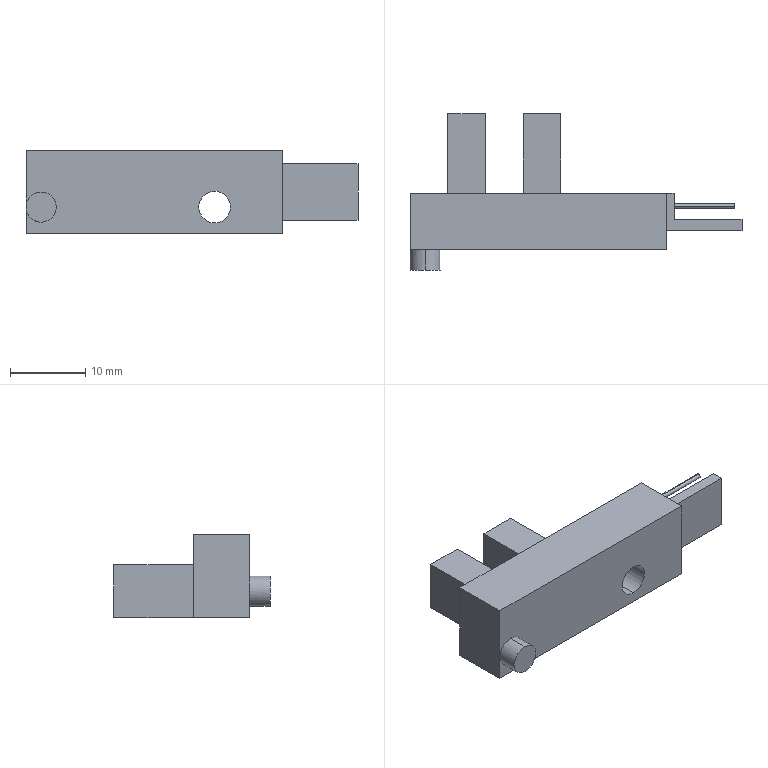Part | SolidWorks | features BaseBody 1 | 1 solid | 34 faces | box 44 x 20.7 x 11 mm | volume 3616 mm3 | plane 24 | cylinder 10 | commonest cylinder face diameters 0.6 x6 4 x2 4.2 x2
STEP:
#1=CARTESIAN_POINT('',(26.,5.78,-2.7));
#2=VERTEX_POINT('',#1);
#3=CARTESIAN_POINT('',(26.,5.78,-3.3));
#4=VERTEX_POINT('',#3);
#5=CARTESIAN_POINT('',(26.,5.78,-3.));
#6=DIRECTION('',(1.,0.,0.));
#7=DIRECTION('',(0.,0.,1.));
#8=AXIS2_PLACEMENT_3D('',#5,#6,#7);
#9=CIRCLE('',#8,0.3);
#10=EDGE_CURVE('',#2,#4,#9,.T.);
#11=ORIENTED_EDGE('',*,*,#10,.T.);
#12=CARTESIAN_POINT('',(26.,5.78,-3.));
#13=DIRECTION('',(1.,0.,0.));
#14=DIRECTION('',(0.,0.,1.));
#15=AXIS2_PLACEMENT_3D('',#12,#13,#14);
#16=CIRCLE('',#15,0.3);
#17=EDGE_CURVE('',#4,#2,#16,.T.);
#18=ORIENTED_EDGE('',*,*,#17,.T.);
#19=EDGE_LOOP('',(#11,#18));
#20=FACE_OUTER_BOUND('',#19,.T.);
#21=CARTESIAN_POINT('',(26.,5.78,-3.));
#22=DIRECTION('',(-1.,0.,0.));
#23=DIRECTION('',(0.,0.,1.));
#24=AXIS2_PLACEMENT_3D('',#21,#22,#23);
#25=PLANE('',#24);
#26=ADVANCED_FACE('',(#20),#25,.F.);
#27=CARTESIAN_POINT('',(18.,5.78,-3.3));
#28=VERTEX_POINT('',#27);
#29=CARTESIAN_POINT('',(26.,5.78,-3.3));
#30=DIRECTION('',(-1.,0.,0.));
#31=VECTOR('',#30,1000.);
#32=LINE('',#29,#31);
#33=EDGE_CURVE('',#4,#28,#32,.T.);
#34=ORIENTED_EDGE('',*,*,#33,.F.);
#35=ORIENTED_EDGE('',*,*,#10,.F.);
#36=CARTESIAN_POINT('',(18.,5.78,-2.7));
#37=VERTEX_POINT('',#36);
#38=CARTESIAN_POINT('',(26.,5.78,-2.7));
#39=DIRECTION('',(-1.,0.,0.));
#40=VECTOR('',#39,1000.);
#41=LINE('',#38,#40);
#42=EDGE_CURVE('',#2,#37,#41,.T.);
#43=ORIENTED_EDGE('',*,*,#42,.T.);
#44=CARTESIAN_POINT('',(18.,5.78,-3.));
#45=DIRECTION('',(1.,0.,0.));
#46=DIRECTION('',(0.,0.,1.));
#47=AXIS2_PLACEMENT_3D('',#44,#45,#46);
#48=CIRCLE('',#47,0.3);
#49=EDGE_CURVE('',#37,#28,#48,.T.);
#50=ORIENTED_EDGE('',*,*,#49,.T.);
#51=EDGE_LOOP('',(#34,#35,#43,#50));
#52=FACE_OUTER_BOUND('',#51,.T.);
#53=CARTESIAN_POINT('',(26.,5.78,-3.));
#54=DIRECTION('',(-1.,0.,0.));
#55=DIRECTION('',(0.,0.,1.));
#56=AXIS2_PLACEMENT_3D('',#53,#54,#55);
#57=CYLINDRICAL_SURFACE('',#56,0.3);
#58=ADVANCED_FACE('',(#52),#57,.T.);
#59=CARTESIAN_POINT('',(26.,5.78,0.3));
#60=VERTEX_POINT('',#59);
#61=CARTESIAN_POINT('',(26.,5.78,-0.3));
#62=VERTEX_POINT('',#61);
#63=CARTESIAN_POINT('',(26.,5.78,0.));
#64=DIRECTION('',(1.,0.,0.));
#65=DIRECTION('',(0.,0.,-1.));
#66=AXIS2_PLACEMENT_3D('',#63,#64,#65);
#67=CIRCLE('',#66,0.3);
#68=EDGE_CURVE('',#60,#62,#67,.T.);
#69=ORIENTED_EDGE('',*,*,#68,.T.);
#70=CARTESIAN_POINT('',(26.,5.78,0.));
#71=DIRECTION('',(1.,0.,0.));
#72=DIRECTION('',(0.,0.,-1.));
#73=AXIS2_PLACEMENT_3D('',#70,#71,#72);
#74=CIRCLE('',#73,0.3);
#75=EDGE_CURVE('',#62,#60,#74,.T.);
#76=ORIENTED_EDGE('',*,*,#75,.T.);
#77=EDGE_LOOP('',(#69,#76));
#78=FACE_OUTER_BOUND('',#77,.T.);
#79=CARTESIAN_POINT('',(26.,5.78,0.));
#80=DIRECTION('',(1.,0.,0.));
#81=DIRECTION('',(0.,1.,0.));
#82=AXIS2_PLACEMENT_3D('',#79,#80,#81);
#83=PLANE('',#82);
#84=ADVANCED_FACE('',(#78),#83,.T.);
#85=CARTESIAN_POINT('',(18.,5.78,-0.3));
#86=VERTEX_POINT('',#85);
#87=CARTESIAN_POINT('',(26.,5.78,-0.3));
#88=DIRECTION('',(-1.,0.,0.));
#89=VECTOR('',#88,1000.);
#90=LINE('',#87,#89);
#91=EDGE_CURVE('',#62,#86,#90,.T.);
#92=ORIENTED_EDGE('',*,*,#91,.F.);
#93=ORIENTED_EDGE('',*,*,#68,.F.);
#94=CARTESIAN_POINT('',(18.,5.78,0.3));
#95=VERTEX_POINT('',#94);
#96=CARTESIAN_POINT('',(26.,5.78,0.3));
#97=DIRECTION('',(-1.,0.,0.));
#98=VECTOR('',#97,1000.);
#99=LINE('',#96,#98);
#100=EDGE_CURVE('',#60,#95,#99,.T.);
#101=ORIENTED_EDGE('',*,*,#100,.T.);
#102=CARTESIAN_POINT('',(18.,5.78,0.));
#103=DIRECTION('',(1.,0.,0.));
#104=DIRECTION('',(0.,0.,1.));
#105=AXIS2_PLACEMENT_3D('',#102,#103,#104);
#106=CIRCLE('',#105,0.3);
#107=EDGE_CURVE('',#95,#86,#106,.T.);
#108=ORIENTED_EDGE('',*,*,#107,.T.);
#109=EDGE_LOOP('',(#92,#93,#101,#108));
#110=FACE_OUTER_BOUND('',#109,.T.);
#111=CARTESIAN_POINT('',(26.,5.78,0.));
#112=DIRECTION('',(-1.,0.,0.));
#113=DIRECTION('',(0.,0.,1.));
#114=AXIS2_PLACEMENT_3D('',#111,#112,#113);
#115=CYLINDRICAL_SURFACE('',#114,0.3);
#116=ADVANCED_FACE('',(#110),#115,.T.);
#117=CARTESIAN_POINT('',(26.,5.78,3.3));
#118=VERTEX_POINT('',#117);
#119=CARTESIAN_POINT('',(26.,5.78,2.7));
#120=VERTEX_POINT('',#119);
#121=CARTESIAN_POINT('',(26.,5.78,3.));
#122=DIRECTION('',(1.,0.,0.));
#123=DIRECTION('',(0.,0.,-1.));
#124=AXIS2_PLACEMENT_3D('',#121,#122,#123);
#125=CIRCLE('',#124,0.3);
#126=EDGE_CURVE('',#118,#120,#125,.T.);
#127=ORIENTED_EDGE('',*,*,#126,.T.);
#128=CARTESIAN_POINT('',(26.,5.78,3.));
#129=DIRECTION('',(1.,0.,0.));
#130=DIRECTION('',(0.,0.,-1.));
#131=AXIS2_PLACEMENT_3D('',#128,#129,#130);
#132=CIRCLE('',#131,0.3);
#133=EDGE_CURVE('',#120,#118,#132,.T.);
#134=ORIENTED_EDGE('',*,*,#133,.T.);
#135=EDGE_LOOP('',(#127,#134));
#136=FACE_OUTER_BOUND('',#135,.T.);
#137=CARTESIAN_POINT('',(26.,5.78,3.));
#138=DIRECTION('',(1.,0.,0.));
#139=DIRECTION('',(0.,1.,0.));
#140=AXIS2_PLACEMENT_3D('',#137,#138,#139);
#141=PLANE('',#140);
#142=ADVANCED_FACE('',(#136),#141,.T.);
#143=CARTESIAN_POINT('',(18.,5.78,2.7));
#144=VERTEX_POINT('',#143);
#145=CARTESIAN_POINT('',(26.,5.78,2.7));
#146=DIRECTION('',(-1.,0.,0.));
#147=VECTOR('',#146,1000.);
#148=LINE('',#145,#147);
#149=EDGE_CURVE('',#120,#144,#148,.T.);
#150=ORIENTED_EDGE('',*,*,#149,.F.);
#151=ORIENTED_EDGE('',*,*,#126,.F.);
#152=CARTESIAN_POINT('',(18.,5.78,3.3));
#153=VERTEX_POINT('',#152);
#154=CARTESIAN_POINT('',(26.,5.78,3.3));
#155=DIRECTION('',(-1.,0.,0.));
#156=VECTOR('',#155,1000.);
#157=LINE('',#154,#156);
#158=EDGE_CURVE('',#118,#153,#157,.T.);
#159=ORIENTED_EDGE('',*,*,#158,.T.);
#160=CARTESIAN_POINT('',(18.,5.78,3.));
#161=DIRECTION('',(1.,0.,0.));
#162=DIRECTION('',(0.,0.,1.));
#163=AXIS2_PLACEMENT_3D('',#160,#161,#162);
#164=CIRCLE('',#163,0.3);
#165=EDGE_CURVE('',#153,#144,#164,.T.);
#166=ORIENTED_EDGE('',*,*,#165,.T.);
#167=EDGE_LOOP('',(#150,#151,#159,#166));
#168=FACE_OUTER_BOUND('',#167,.T.);
#169=CARTESIAN_POINT('',(26.,5.78,3.));
#170=DIRECTION('',(-1.,0.,0.));
#171=DIRECTION('',(0.,0.,1.));
#172=AXIS2_PLACEMENT_3D('',#169,#170,#171);
#173=CYLINDRICAL_SURFACE('',#172,0.3);
#174=ADVANCED_FACE('',(#168),#173,.T.);
#175=CARTESIAN_POINT('',(27.,4.,3.75));
#176=VERTEX_POINT('',#175);
#177=CARTESIAN_POINT('',(27.,4.,-3.75));
#178=VERTEX_POINT('',#177);
#179=CARTESIAN_POINT('',(27.,4.,-3.75));
#180=DIRECTION('',(0.,0.,-1.));
#181=VECTOR('',#180,1000.);
#182=LINE('',#179,#181);
#183=EDGE_CURVE('',#176,#178,#182,.T.);
#184=ORIENTED_EDGE('',*,*,#183,.T.);
#185=CARTESIAN_POINT('',(18.,4.,-3.75));
#186=VERTEX_POINT('',#185);
#187=CARTESIAN_POINT('',(27.,4.,-3.75));
#188=DIRECTION('',(-1.,0.,0.));
#189=VECTOR('',#188,1000.);
#190=LINE('',#187,#189);
#191=EDGE_CURVE('',#178,#186,#190,.T.);
#192=ORIENTED_EDGE('',*,*,#191,.T.);
#193=CARTESIAN_POINT('',(18.,4.,3.75));
#194=VERTEX_POINT('',#193);
#195=CARTESIAN_POINT('',(18.,4.,-3.75));
#196=DIRECTION('',(0.,0.,1.));
#197=VECTOR('',#196,1000.);
#198=LINE('',#195,#197);
#199=EDGE_CURVE('',#186,#194,#198,.T.);
#200=ORIENTED_EDGE('',*,*,#199,.T.);
#201=CARTESIAN_POINT('',(27.,4.,3.75));
#202=DIRECTION('',(1.,0.,0.));
#203=VECTOR('',#202,1000.);
#204=LINE('',#201,#203);
#205=EDGE_CURVE('',#194,#176,#204,.T.);
#206=ORIENTED_EDGE('',*,*,#205,.T.);
#207=EDGE_LOOP('',(#184,#192,#200,#206));
#208=FACE_OUTER_BOUND('',#207,.T.);
#209=CARTESIAN_POINT('',(0.,4.,0.));
#210=DIRECTION('',(0.,-1.,0.));
#211=DIRECTION('',(0.,0.,-1.));
#212=AXIS2_PLACEMENT_3D('',#209,#210,#211);
#213=PLANE('',#212);
#214=ADVANCED_FACE('',(#208),#213,.F.);
#215=ORIENTED_EDGE('',*,*,#165,.F.);
#216=CARTESIAN_POINT('',(18.,5.78,3.));
#217=DIRECTION('',(1.,0.,0.));
#218=DIRECTION('',(0.,0.,1.));
#219=AXIS2_PLACEMENT_3D('',#216,#217,#218);
#220=CIRCLE('',#219,0.3);
#221=EDGE_CURVE('',#144,#153,#220,.T.);
#222=ORIENTED_EDGE('',*,*,#221,.F.);
#223=EDGE_LOOP('',(#215,#222));
#224=FACE_BOUND('',#223,.T.);
#225=ORIENTED_EDGE('',*,*,#107,.F.);
#226=CARTESIAN_POINT('',(18.,5.78,0.));
#227=DIRECTION('',(1.,0.,0.));
#228=DIRECTION('',(0.,0.,1.));
#229=AXIS2_PLACEMENT_3D('',#226,#227,#228);
#230=CIRCLE('',#229,0.3);
#231=EDGE_CURVE('',#86,#95,#230,.T.);
#232=ORIENTED_EDGE('',*,*,#231,.F.);
#233=EDGE_LOOP('',(#225,#232));
#234=FACE_BOUND('',#233,.T.);
#235=ORIENTED_EDGE('',*,*,#49,.F.);
#236=CARTESIAN_POINT('',(18.,5.78,-3.));
#237=DIRECTION('',(1.,0.,0.));
#238=DIRECTION('',(0.,0.,1.));
#239=AXIS2_PLACEMENT_3D('',#236,#237,#238);
#240=CIRCLE('',#239,0.3);
#241=EDGE_CURVE('',#28,#37,#240,.T.);
#242=ORIENTED_EDGE('',*,*,#241,.F.);
#243=EDGE_LOOP('',(#235,#242));
#244=FACE_BOUND('',#243,.T.);
#245=CARTESIAN_POINT('',(18.,7.5,-3.75));
#246=VERTEX_POINT('',#245);
#247=CARTESIAN_POINT('',(18.,7.5,3.75));
#248=VERTEX_POINT('',#247);
#249=CARTESIAN_POINT('',(18.,7.5,-3.75));
#250=DIRECTION('',(0.,0.,1.));
#251=VECTOR('',#250,1000.);
#252=LINE('',#249,#251);
#253=EDGE_CURVE('',#246,#248,#252,.T.);
#254=ORIENTED_EDGE('',*,*,#253,.T.);
#255=CARTESIAN_POINT('',(18.,4.,3.75));
#256=DIRECTION('',(0.,1.,0.));
#257=VECTOR('',#256,1000.);
#258=LINE('',#255,#257);
#259=EDGE_CURVE('',#194,#248,#258,.T.);
#260=ORIENTED_EDGE('',*,*,#259,.F.);
#261=ORIENTED_EDGE('',*,*,#199,.F.);
#262=CARTESIAN_POINT('',(18.,4.,-3.75));
#263=DIRECTION('',(0.,1.,0.));
#264=VECTOR('',#263,1000.);
#265=LINE('',#262,#264);
#266=EDGE_CURVE('',#186,#246,#265,.T.);
#267=ORIENTED_EDGE('',*,*,#266,.T.);
#268=EDGE_LOOP('',(#254,#260,#261,#267));
#269=FACE_OUTER_BOUND('',#268,.T.);
#270=CARTESIAN_POINT('',(18.,4.,-3.75));
#271=DIRECTION('',(-1.,0.,0.));
#272=DIRECTION('',(0.,0.,1.));
#273=AXIS2_PLACEMENT_3D('',#270,#271,#272);
#274=PLANE('',#273);
#275=ADVANCED_FACE('',(#224,#234,#244,#269),#274,.F.);
#276=ORIENTED_EDGE('',*,*,#183,.F.);
#277=CARTESIAN_POINT('',(27.,2.5,3.75));
#278=VERTEX_POINT('',#277);
#279=CARTESIAN_POINT('',(27.,7.5,3.75));
#280=DIRECTION('',(0.,-1.,0.));
#281=VECTOR('',#280,1000.);
#282=LINE('',#279,#281);
#283=EDGE_CURVE('',#176,#278,#282,.T.);
#284=ORIENTED_EDGE('',*,*,#283,.T.);
#285=CARTESIAN_POINT('',(27.,2.5,-3.75));
#286=VERTEX_POINT('',#285);
#287=CARTESIAN_POINT('',(27.,2.5,3.75));
#288=DIRECTION('',(0.,0.,-1.));
#289=VECTOR('',#288,1000.);
#290=LINE('',#287,#289);
#291=EDGE_CURVE('',#278,#286,#290,.T.);
#292=ORIENTED_EDGE('',*,*,#291,.T.);
#293=CARTESIAN_POINT('',(27.,7.5,-3.75));
#294=DIRECTION('',(0.,1.,0.));
#295=VECTOR('',#294,1000.);
#296=LINE('',#293,#295);
#297=EDGE_CURVE('',#286,#178,#296,.T.);
#298=ORIENTED_EDGE('',*,*,#297,.T.);
#299=EDGE_LOOP('',(#276,#284,#292,#298));
#300=FACE_OUTER_BOUND('',#299,.T.);
#301=CARTESIAN_POINT('',(27.,0.,0.));
#302=DIRECTION('',(1.,0.,0.));
#303=DIRECTION('',(0.,1.,0.));
#304=AXIS2_PLACEMENT_3D('',#301,#302,#303);
#305=PLANE('',#304);
#306=ADVANCED_FACE('',(#300),#305,.T.);
#307=CARTESIAN_POINT('',(17.,7.5,-3.75));
#308=VERTEX_POINT('',#307);
#309=CARTESIAN_POINT('',(27.,7.5,-3.75));
#310=DIRECTION('',(-1.,0.,0.));
#311=VECTOR('',#310,1000.);
#312=LINE('',#309,#311);
#313=EDGE_CURVE('',#246,#308,#312,.T.);
#314=ORIENTED_EDGE('',*,*,#313,.F.);
#315=ORIENTED_EDGE('',*,*,#266,.F.);
#316=ORIENTED_EDGE('',*,*,#191,.F.);
#317=ORIENTED_EDGE('',*,*,#297,.F.);
#318=CARTESIAN_POINT('',(17.,2.5,-3.75));
#319=VERTEX_POINT('',#318);
#320=CARTESIAN_POINT('',(27.,2.5,-3.75));
#321=DIRECTION('',(-1.,0.,0.));
#322=VECTOR('',#321,1000.);
#323=LINE('',#320,#322);
#324=EDGE_CURVE('',#286,#319,#323,.T.);
#325=ORIENTED_EDGE('',*,*,#324,.T.);
#326=CARTESIAN_POINT('',(17.,7.5,-3.75));
#327=DIRECTION('',(0.,1.,0.));
#328=VECTOR('',#327,1000.);
#329=LINE('',#326,#328);
#330=EDGE_CURVE('',#319,#308,#329,.T.);
#331=ORIENTED_EDGE('',*,*,#330,.T.);
#332=EDGE_LOOP('',(#314,#315,#316,#317,#325,#331));
#333=FACE_OUTER_BOUND('',#332,.T.);
#334=CARTESIAN_POINT('',(27.,7.5,-3.75));
#335=DIRECTION('',(0.,0.,1.));
#336=DIRECTION('',(0.,-1.,0.));
#337=AXIS2_PLACEMENT_3D('',#334,#335,#336);
#338=PLANE('',#337);
#339=ADVANCED_FACE('',(#333),#338,.F.);
#340=CARTESIAN_POINT('',(17.,2.5,3.75));
#341=VERTEX_POINT('',#340);
#342=CARTESIAN_POINT('',(17.,2.5,3.75));
#343=DIRECTION('',(0.,0.,-1.));
#344=VECTOR('',#343,1000.);
#345=LINE('',#342,#344);
#346=EDGE_CURVE('',#341,#319,#345,.T.);
#347=ORIENTED_EDGE('',*,*,#346,.T.);
#348=ORIENTED_EDGE('',*,*,#324,.F.);
#349=ORIENTED_EDGE('',*,*,#291,.F.);
#350=CARTESIAN_POINT('',(27.,2.5,3.75));
#351=DIRECTION('',(-1.,0.,0.));
#352=VECTOR('',#351,1000.);
#353=LINE('',#350,#352);
#354=EDGE_CURVE('',#278,#341,#353,.T.);
#355=ORIENTED_EDGE('',*,*,#354,.T.);
#356=EDGE_LOOP('',(#347,#348,#349,#355));
#357=FACE_OUTER_BOUND('',#356,.T.);
#358=CARTESIAN_POINT('',(27.,2.5,3.75));
#359=DIRECTION('',(0.,1.,0.));
#360=DIRECTION('',(1.,0.,0.));
#361=AXIS2_PLACEMENT_3D('',#358,#359,#360);
#362=PLANE('',#361);
#363=ADVANCED_FACE('',(#357),#362,.F.);
#364=ORIENTED_EDGE('',*,*,#205,.F.);
#365=ORIENTED_EDGE('',*,*,#259,.T.);
#366=CARTESIAN_POINT('',(17.,7.5,3.75));
#367=VERTEX_POINT('',#366);
#368=CARTESIAN_POINT('',(27.,7.5,3.75));
#369=DIRECTION('',(-1.,0.,0.));
#370=VECTOR('',#369,1000.);
#371=LINE('',#368,#370);
#372=EDGE_CURVE('',#248,#367,#371,.T.);
#373=ORIENTED_EDGE('',*,*,#372,.T.);
#374=CARTESIAN_POINT('',(17.,7.5,3.75));
#375=DIRECTION('',(0.,-1.,0.));
#376=VECTOR('',#375,1000.);
#377=LINE('',#374,#376);
#378=EDGE_CURVE('',#367,#341,#377,.T.);
#379=ORIENTED_EDGE('',*,*,#378,.T.);
#380=ORIENTED_EDGE('',*,*,#354,.F.);
#381=ORIENTED_EDGE('',*,*,#283,.F.);
#382=EDGE_LOOP('',(#364,#365,#373,#379,#380,#381));
#383=FACE_OUTER_BOUND('',#382,.T.);
#384=CARTESIAN_POINT('',(27.,7.5,3.75));
#385=DIRECTION('',(0.,0.,-1.));
#386=DIRECTION('',(-1.,0.,0.));
#387=AXIS2_PLACEMENT_3D('',#384,#385,#386);
#388=PLANE('',#387);
#389=ADVANCED_FACE('',(#383),#388,.F.);
#390=CARTESIAN_POINT('',(-2.,18.,-5.5));
#391=VERTEX_POINT('',#390);
#392=CARTESIAN_POINT('',(-2.,18.,1.5));
#393=VERTEX_POINT('',#392);
#394=CARTESIAN_POINT('',(-2.,18.,-5.5));
#395=DIRECTION('',(0.,0.,1.));
#396=VECTOR('',#395,1000.);
#397=LINE('',#394,#396);
#398=EDGE_CURVE('',#391,#393,#397,.T.);
#399=ORIENTED_EDGE('',*,*,#398,.T.);
#400=CARTESIAN_POINT('',(3.,18.,1.5));
#401=VERTEX_POINT('',#400);
#402=CARTESIAN_POINT('',(-2.,18.,1.5));
#403=DIRECTION('',(1.,0.,0.));
#404=VECTOR('',#403,1000.);
#405=LINE('',#402,#404);
#406=EDGE_CURVE('',#393,#401,#405,.T.);
#407=ORIENTED_EDGE('',*,*,#406,.T.);
#408=CARTESIAN_POINT('',(3.,18.,-5.5));
#409=VERTEX_POINT('',#408);
#410=CARTESIAN_POINT('',(3.,18.,-5.5));
#411=DIRECTION('',(0.,0.,-1.));
#412=VECTOR('',#411,1000.);
#413=LINE('',#410,#412);
#414=EDGE_CURVE('',#401,#409,#413,.T.);
#415=ORIENTED_EDGE('',*,*,#414,.T.);
#416=CARTESIAN_POINT('',(-2.,18.,-5.5));
#417=DIRECTION('',(-1.,0.,0.));
#418=VECTOR('',#417,1000.);
#419=LINE('',#416,#418);
#420=EDGE_CURVE('',#409,#391,#419,.T.);
#421=ORIENTED_EDGE('',*,*,#420,.T.);
#422=EDGE_LOOP('',(#399,#407,#415,#421));
#423=FACE_OUTER_BOUND('',#422,.T.);
#424=CARTESIAN_POINT('',(0.,18.,0.));
#425=DIRECTION('',(0.,1.,0.));
#426=DIRECTION('',(1.,0.,0.));
#427=AXIS2_PLACEMENT_3D('',#424,#425,#426);
#428=PLANE('',#427);
#429=ADVANCED_FACE('',(#423),#428,.T.);
#430=CARTESIAN_POINT('',(3.,7.5,1.5));
#431=VERTEX_POINT('',#430);
#432=CARTESIAN_POINT('',(3.,7.5,-5.5));
#433=VERTEX_POINT('',#432);
#434=CARTESIAN_POINT('',(3.,7.5,-5.5));
#435=DIRECTION('',(0.,0.,-1.));
#436=VECTOR('',#435,1000.);
#437=LINE('',#434,#436);
#438=EDGE_CURVE('',#431,#433,#437,.T.);
#439=ORIENTED_EDGE('',*,*,#438,.T.);
#440=CARTESIAN_POINT('',(3.,18.,-5.5));
#441=DIRECTION('',(0.,-1.,0.));
#442=VECTOR('',#441,1000.);
#443=LINE('',#440,#442);
#444=EDGE_CURVE('',#409,#433,#443,.T.);
#445=ORIENTED_EDGE('',*,*,#444,.F.);
#446=ORIENTED_EDGE('',*,*,#414,.F.);
#447=CARTESIAN_POINT('',(3.,18.,1.5));
#448=DIRECTION('',(0.,-1.,0.));
#449=VECTOR('',#448,1000.);
#450=LINE('',#447,#449);
#451=EDGE_CURVE('',#401,#431,#450,.T.);
#452=ORIENTED_EDGE('',*,*,#451,.T.);
#453=EDGE_LOOP('',(#439,#445,#446,#452));
#454=FACE_OUTER_BOUND('',#453,.T.);
#455=CARTESIAN_POINT('',(3.,18.,-5.5));
#456=DIRECTION('',(-1.,0.,0.));
#457=DIRECTION('',(0.,1.,0.));
#458=AXIS2_PLACEMENT_3D('',#455,#456,#457);
#459=PLANE('',#458);
#460=ADVANCED_FACE('',(#454),#459,.F.);
#461=CARTESIAN_POINT('',(-2.,7.5,1.5));
#462=VERTEX_POINT('',#461);
#463=CARTESIAN_POINT('',(-2.,7.5,1.5));
#464=DIRECTION('',(1.,0.,0.));
#465=VECTOR('',#464,1000.);
#466=LINE('',#463,#465);
#467=EDGE_CURVE('',#462,#431,#466,.T.);
#468=ORIENTED_EDGE('',*,*,#467,.T.);
#469=ORIENTED_EDGE('',*,*,#451,.F.);
#470=ORIENTED_EDGE('',*,*,#406,.F.);
#471=CARTESIAN_POINT('',(-2.,18.,1.5));
#472=DIRECTION('',(0.,-1.,0.));
#473=VECTOR('',#472,1000.);
#474=LINE('',#471,#473);
#475=EDGE_CURVE('',#393,#462,#474,.T.);
#476=ORIENTED_EDGE('',*,*,#475,.T.);
#477=EDGE_LOOP('',(#468,#469,#470,#476));
#478=FACE_OUTER_BOUND('',#477,.T.);
#479=CARTESIAN_POINT('',(-2.,18.,1.5));
#480=DIRECTION('',(0.,0.,-1.));
#481=DIRECTION('',(0.,-1.,0.));
#482=AXIS2_PLACEMENT_3D('',#479,#480,#481);
#483=PLANE('',#482);
#484=ADVANCED_FACE('',(#478),#483,.F.);
#485=CARTESIAN_POINT('',(-2.,7.5,-5.5));
#486=VERTEX_POINT('',#485);
#487=CARTESIAN_POINT('',(-2.,7.5,-5.5));
#488=DIRECTION('',(0.,0.,1.));
#489=VECTOR('',#488,1000.);
#490=LINE('',#487,#489);
#491=EDGE_CURVE('',#486,#462,#490,.T.);
#492=ORIENTED_EDGE('',*,*,#491,.T.);
#493=ORIENTED_EDGE('',*,*,#475,.F.);
#494=ORIENTED_EDGE('',*,*,#398,.F.);
#495=CARTESIAN_POINT('',(-2.,18.,-5.5));
#496=DIRECTION('',(0.,-1.,0.));
#497=VECTOR('',#496,1000.);
#498=LINE('',#495,#497);
#499=EDGE_CURVE('',#391,#486,#498,.T.);
#500=ORIENTED_EDGE('',*,*,#499,.T.);
#501=EDGE_LOOP('',(#492,#493,#494,#500));
#502=FACE_OUTER_BOUND('',#501,.T.);
#503=CARTESIAN_POINT('',(-2.,18.,-5.5));
#504=DIRECTION('',(1.,0.,0.));
#505=DIRECTION('',(0.,0.,-1.));
#506=AXIS2_PLACEMENT_3D('',#503,#504,#505);
#507=PLANE('',#506);
#508=ADVANCED_FACE('',(#502),#507,.F.);
#509=CARTESIAN_POINT('',(-12.,18.,-5.5));
#510=VERTEX_POINT('',#509);
#511=CARTESIAN_POINT('',(-12.,18.,1.5));
#512=VERTEX_POINT('',#511);
#513=CARTESIAN_POINT('',(-12.,18.,-5.5));
#514=DIRECTION('',(0.,0.,1.));
#515=VECTOR('',#514,1000.);
#516=LINE('',#513,#515);
#517=EDGE_CURVE('',#510,#512,#516,.T.);
#518=ORIENTED_EDGE('',*,*,#517,.T.);
#519=CARTESIAN_POINT('',(-7.,18.,1.5));
#520=VERTEX_POINT('',#519);
#521=CARTESIAN_POINT('',(-12.,18.,1.5));
#522=DIRECTION('',(1.,0.,0.));
#523=VECTOR('',#522,1000.);
#524=LINE('',#521,#523);
#525=EDGE_CURVE('',#512,#520,#524,.T.);
#526=ORIENTED_EDGE('',*,*,#525,.T.);
#527=CARTESIAN_POINT('',(-7.,18.,-5.5));
#528=VERTEX_POINT('',#527);
#529=CARTESIAN_POINT('',(-7.,18.,-5.5));
#530=DIRECTION('',(0.,0.,-1.));
#531=VECTOR('',#530,1000.);
#532=LINE('',#529,#531);
#533=EDGE_CURVE('',#520,#528,#532,.T.);
#534=ORIENTED_EDGE('',*,*,#533,.T.);
#535=CARTESIAN_POINT('',(-12.,18.,-5.5));
#536=DIRECTION('',(-1.,0.,0.));
#537=VECTOR('',#536,1000.);
#538=LINE('',#535,#537);
#539=EDGE_CURVE('',#528,#510,#538,.T.);
#540=ORIENTED_EDGE('',*,*,#539,.T.);
#541=EDGE_LOOP('',(#518,#526,#534,#540));
#542=FACE_OUTER_BOUND('',#541,.T.);
#543=CARTESIAN_POINT('',(0.,18.,0.));
#544=DIRECTION('',(0.,1.,0.));
#545=DIRECTION('',(1.,0.,0.));
#546=AXIS2_PLACEMENT_3D('',#543,#544,#545);
#547=PLANE('',#546);
#548=ADVANCED_FACE('',(#542),#547,.T.);
#549=CARTESIAN_POINT('',(-7.,7.5,1.5));
#550=VERTEX_POINT('',#549);
#551=CARTESIAN_POINT('',(-7.,7.5,-5.5));
#552=VERTEX_POINT('',#551);
#553=CARTESIAN_POINT('',(-7.,7.5,-5.5));
#554=DIRECTION('',(0.,0.,-1.));
#555=VECTOR('',#554,1000.);
#556=LINE('',#553,#555);
#557=EDGE_CURVE('',#550,#552,#556,.T.);
#558=ORIENTED_EDGE('',*,*,#557,.T.);
#559=CARTESIAN_POINT('',(-7.,18.,-5.5));
#560=DIRECTION('',(0.,-1.,0.));
#561=VECTOR('',#560,1000.);
#562=LINE('',#559,#561);
#563=EDGE_CURVE('',#528,#552,#562,.T.);
#564=ORIENTED_EDGE('',*,*,#563,.F.);
#565=ORIENTED_EDGE('',*,*,#533,.F.);
#566=CARTESIAN_POINT('',(-7.,18.,1.5));
#567=DIRECTION('',(0.,-1.,0.));
#568=VECTOR('',#567,1000.);
#569=LINE('',#566,#568);
#570=EDGE_CURVE('',#520,#550,#569,.T.);
#571=ORIENTED_EDGE('',*,*,#570,.T.);
#572=EDGE_LOOP('',(#558,#564,#565,#571));
#573=FACE_OUTER_BOUND('',#572,.T.);
#574=CARTESIAN_POINT('',(-7.,18.,-5.5));
#575=DIRECTION('',(-1.,0.,0.));
#576=DIRECTION('',(0.,1.,0.));
#577=AXIS2_PLACEMENT_3D('',#574,#575,#576);
#578=PLANE('',#577);
#579=ADVANCED_FACE('',(#573),#578,.F.);
#580=CARTESIAN_POINT('',(-12.,7.5,1.5));
#581=VERTEX_POINT('',#580);
#582=CARTESIAN_POINT('',(-12.,7.5,1.5));
#583=DIRECTION('',(1.,0.,0.));
#584=VECTOR('',#583,1000.);
#585=LINE('',#582,#584);
#586=EDGE_CURVE('',#581,#550,#585,.T.);
#587=ORIENTED_EDGE('',*,*,#586,.T.);
#588=ORIENTED_EDGE('',*,*,#570,.F.);
#589=ORIENTED_EDGE('',*,*,#525,.F.);
#590=CARTESIAN_POINT('',(-12.,18.,1.5));
#591=DIRECTION('',(0.,-1.,0.));
#592=VECTOR('',#591,1000.);
#593=LINE('',#590,#592);
#594=EDGE_CURVE('',#512,#581,#593,.T.);
#595=ORIENTED_EDGE('',*,*,#594,.T.);
#596=EDGE_LOOP('',(#587,#588,#589,#595));
#597=FACE_OUTER_BOUND('',#596,.T.);
#598=CARTESIAN_POINT('',(-12.,18.,1.5));
#599=DIRECTION('',(0.,0.,-1.));
#600=DIRECTION('',(0.,-1.,0.));
#601=AXIS2_PLACEMENT_3D('',#598,#599,#600);
#602=PLANE('',#601);
#603=ADVANCED_FACE('',(#597),#602,.F.);
#604=CARTESIAN_POINT('',(-12.,7.5,-5.5));
#605=VERTEX_POINT('',#604);
#606=CARTESIAN_POINT('',(-12.,7.5,-5.5));
#607=DIRECTION('',(0.,0.,1.));
#608=VECTOR('',#607,1000.);
#609=LINE('',#606,#608);
#610=EDGE_CURVE('',#605,#581,#609,.T.);
#611=ORIENTED_EDGE('',*,*,#610,.T.);
#612=ORIENTED_EDGE('',*,*,#594,.F.);
#613=ORIENTED_EDGE('',*,*,#517,.F.);
#614=CARTESIAN_POINT('',(-12.,18.,-5.5));
#615=DIRECTION('',(0.,-1.,0.));
#616=VECTOR('',#615,1000.);
#617=LINE('',#614,#616);
#618=EDGE_CURVE('',#510,#605,#617,.T.);
#619=ORIENTED_EDGE('',*,*,#618,.T.);
#620=EDGE_LOOP('',(#611,#612,#613,#619));
#621=FACE_OUTER_BOUND('',#620,.T.);
#622=CARTESIAN_POINT('',(-12.,18.,-5.5));
#623=DIRECTION('',(1.,0.,0.));
#624=DIRECTION('',(0.,1.,0.));
#625=AXIS2_PLACEMENT_3D('',#622,#623,#624);
#626=PLANE('',#625);
#627=ADVANCED_FACE('',(#621),#626,.F.);
#628=CARTESIAN_POINT('',(8.,7.5,0.1));
#629=VERTEX_POINT('',#628);
#630=CARTESIAN_POINT('',(8.,0.,0.1));
#631=VERTEX_POINT('',#630);
#632=CARTESIAN_POINT('',(8.,7.5,0.1));
#633=DIRECTION('',(0.,-1.,0.));
#634=VECTOR('',#633,1000.);
#635=LINE('',#632,#634);
#636=EDGE_CURVE('',#629,#631,#635,.T.);
#637=ORIENTED_EDGE('',*,*,#636,.F.);
#638=CARTESIAN_POINT('',(8.,7.5,-4.1));
#639=VERTEX_POINT('',#638);
#640=CARTESIAN_POINT('',(8.,7.5,-2.));
#641=DIRECTION('',(0.,-1.,0.));
#642=DIRECTION('',(0.,0.,-1.));
#643=AXIS2_PLACEMENT_3D('',#640,#641,#642);
#644=CIRCLE('',#643,2.1);
#645=EDGE_CURVE('',#639,#629,#644,.T.);
#646=ORIENTED_EDGE('',*,*,#645,.F.);
#647=CARTESIAN_POINT('',(8.,0.,-4.1));
#648=VERTEX_POINT('',#647);
#649=CARTESIAN_POINT('',(8.,7.5,-4.1));
#650=DIRECTION('',(0.,-1.,0.));
#651=VECTOR('',#650,1000.);
#652=LINE('',#649,#651);
#653=EDGE_CURVE('',#639,#648,#652,.T.);
#654=ORIENTED_EDGE('',*,*,#653,.T.);
#655=CARTESIAN_POINT('',(8.,0.,-2.));
#656=DIRECTION('',(0.,-1.,0.));
#657=DIRECTION('',(0.,0.,-1.));
#658=AXIS2_PLACEMENT_3D('',#655,#656,#657);
#659=CIRCLE('',#658,2.1);
#660=EDGE_CURVE('',#648,#631,#659,.T.);
#661=ORIENTED_EDGE('',*,*,#660,.T.);
#662=EDGE_LOOP('',(#637,#646,#654,#661));
#663=FACE_OUTER_BOUND('',#662,.T.);
#664=CARTESIAN_POINT('',(8.,7.5,-2.));
#665=DIRECTION('',(0.,-1.,0.));
#666=DIRECTION('',(0.,0.,-1.));
#667=AXIS2_PLACEMENT_3D('',#664,#665,#666);
#668=CYLINDRICAL_SURFACE('',#667,2.1);
#669=ADVANCED_FACE('',(#663),#668,.F.);
#670=CARTESIAN_POINT('',(-15.,-2.7,0.));
#671=VERTEX_POINT('',#670);
#672=CARTESIAN_POINT('',(-15.,-2.7,-4.));
#673=VERTEX_POINT('',#672);
#674=CARTESIAN_POINT('',(-15.,-2.7,-2.));
#675=DIRECTION('',(0.,-1.,0.));
#676=DIRECTION('',(0.,0.,-1.));
#677=AXIS2_PLACEMENT_3D('',#674,#675,#676);
#678=CIRCLE('',#677,2.);
#679=EDGE_CURVE('',#671,#673,#678,.T.);
#680=ORIENTED_EDGE('',*,*,#679,.T.);
#681=CARTESIAN_POINT('',(-15.,-2.7,-2.));
#682=DIRECTION('',(0.,-1.,0.));
#683=DIRECTION('',(0.,0.,-1.));
#684=AXIS2_PLACEMENT_3D('',#681,#682,#683);
#685=CIRCLE('',#684,2.);
#686=EDGE_CURVE('',#673,#671,#685,.T.);
#687=ORIENTED_EDGE('',*,*,#686,.T.);
#688=EDGE_LOOP('',(#680,#687));
#689=FACE_OUTER_BOUND('',#688,.T.);
#690=CARTESIAN_POINT('',(-15.,-2.7,-2.));
#691=DIRECTION('',(0.,-1.,0.));
#692=DIRECTION('',(0.,0.,-1.));
#693=AXIS2_PLACEMENT_3D('',#690,#691,#692);
#694=PLANE('',#693);
#695=ADVANCED_FACE('',(#689),#694,.T.);
#696=CARTESIAN_POINT('',(-15.,0.,-4.));
#697=VERTEX_POINT('',#696);
#698=CARTESIAN_POINT('',(-15.,-2.7,-4.));
#699=DIRECTION('',(0.,1.,0.));
#700=VECTOR('',#699,1000.);
#701=LINE('',#698,#700);
#702=EDGE_CURVE('',#673,#697,#701,.T.);
#703=ORIENTED_EDGE('',*,*,#702,.F.);
#704=ORIENTED_EDGE('',*,*,#679,.F.);
#705=CARTESIAN_POINT('',(-15.,0.,0.));
#706=VERTEX_POINT('',#705);
#707=CARTESIAN_POINT('',(-15.,-2.7,0.));
#708=DIRECTION('',(0.,1.,0.));
#709=VECTOR('',#708,1000.);
#710=LINE('',#707,#709);
#711=EDGE_CURVE('',#671,#706,#710,.T.);
#712=ORIENTED_EDGE('',*,*,#711,.T.);
#713=CARTESIAN_POINT('',(-17.,0.,-2.));
#714=VERTEX_POINT('',#713);
#715=CARTESIAN_POINT('',(-15.,0.,-2.));
#716=DIRECTION('',(0.,-1.,0.));
#717=DIRECTION('',(0.,0.,-1.));
#718=AXIS2_PLACEMENT_3D('',#715,#716,#717);
#719=CIRCLE('',#718,2.);
#720=EDGE_CURVE('',#706,#714,#719,.T.);
#721=ORIENTED_EDGE('',*,*,#720,.T.);
#722=CARTESIAN_POINT('',(-15.,0.,-2.));
#723=DIRECTION('',(0.,-1.,0.));
#724=DIRECTION('',(0.,0.,-1.));
#725=AXIS2_PLACEMENT_3D('',#722,#723,#724);
#726=CIRCLE('',#725,2.);
#727=EDGE_CURVE('',#714,#697,#726,.T.);
#728=ORIENTED_EDGE('',*,*,#727,.T.);
#729=EDGE_LOOP('',(#703,#704,#712,#721,#728));
#730=FACE_OUTER_BOUND('',#729,.T.);
#731=CARTESIAN_POINT('',(-15.,-2.7,-2.));
#732=DIRECTION('',(0.,1.,0.));
#733=DIRECTION('',(0.,0.,1.));
#734=AXIS2_PLACEMENT_3D('',#731,#732,#733);
#735=CYLINDRICAL_SURFACE('',#734,2.);
#736=ADVANCED_FACE('',(#730),#735,.T.);
#737=ORIENTED_EDGE('',*,*,#660,.F.);
#738=CARTESIAN_POINT('',(8.,0.,-2.));
#739=DIRECTION('',(0.,-1.,0.));
#740=DIRECTION('',(0.,0.,-1.));
#741=AXIS2_PLACEMENT_3D('',#738,#739,#740);
#742=CIRCLE('',#741,2.1);
#743=EDGE_CURVE('',#631,#648,#742,.T.);
#744=ORIENTED_EDGE('',*,*,#743,.F.);
#745=EDGE_LOOP('',(#737,#744));
#746=FACE_BOUND('',#745,.T.);
#747=CARTESIAN_POINT('',(-17.,0.,5.5));
#748=VERTEX_POINT('',#747);
#749=CARTESIAN_POINT('',(-17.,0.,-5.5));
#750=DIRECTION('',(0.,0.,1.));
#751=VECTOR('',#750,1000.);
#752=LINE('',#749,#751);
#753=EDGE_CURVE('',#714,#748,#752,.T.);
#754=ORIENTED_EDGE('',*,*,#753,.F.);
#755=ORIENTED_EDGE('',*,*,#720,.F.);
#756=CARTESIAN_POINT('',(-15.,0.,-2.));
#757=DIRECTION('',(0.,-1.,0.));
#758=DIRECTION('',(0.,0.,-1.));
#759=AXIS2_PLACEMENT_3D('',#756,#757,#758);
#760=CIRCLE('',#759,2.);
#761=EDGE_CURVE('',#697,#706,#760,.T.);
#762=ORIENTED_EDGE('',*,*,#761,.F.);
#763=ORIENTED_EDGE('',*,*,#727,.F.);
#764=CARTESIAN_POINT('',(-17.,0.,-5.5));
#765=VERTEX_POINT('',#764);
#766=CARTESIAN_POINT('',(-17.,0.,-5.5));
#767=DIRECTION('',(0.,0.,1.));
#768=VECTOR('',#767,1000.);
#769=LINE('',#766,#768);
#770=EDGE_CURVE('',#765,#714,#769,.T.);
#771=ORIENTED_EDGE('',*,*,#770,.F.);
#772=CARTESIAN_POINT('',(17.,0.,-5.5));
#773=VERTEX_POINT('',#772);
#774=CARTESIAN_POINT('',(-17.,0.,-5.5));
#775=DIRECTION('',(-1.,0.,0.));
#776=VECTOR('',#775,1000.);
#777=LINE('',#774,#776);
#778=EDGE_CURVE('',#773,#765,#777,.T.);
#779=ORIENTED_EDGE('',*,*,#778,.F.);
#780=CARTESIAN_POINT('',(17.,0.,5.5));
#781=VERTEX_POINT('',#780);
#782=CARTESIAN_POINT('',(17.,0.,-5.5));
#783=DIRECTION('',(0.,0.,-1.));
#784=VECTOR('',#783,1000.);
#785=LINE('',#782,#784);
#786=EDGE_CURVE('',#781,#773,#785,.T.);
#787=ORIENTED_EDGE('',*,*,#786,.F.);
#788=CARTESIAN_POINT('',(-17.,0.,5.5));
#789=DIRECTION('',(1.,0.,0.));
#790=VECTOR('',#789,1000.);
#791=LINE('',#788,#790);
#792=EDGE_CURVE('',#748,#781,#791,.T.);
#793=ORIENTED_EDGE('',*,*,#792,.F.);
#794=EDGE_LOOP('',(#754,#755,#762,#763,#771,#779,#787,#793));
#795=FACE_OUTER_BOUND('',#794,.T.);
#796=CARTESIAN_POINT('',(0.,0.,0.));
#797=DIRECTION('',(0.,1.,0.));
#798=DIRECTION('',(1.,0.,0.));
#799=AXIS2_PLACEMENT_3D('',#796,#797,#798);
#800=PLANE('',#799);
#801=ADVANCED_FACE('',(#746,#795),#800,.F.);
#802=ORIENTED_EDGE('',*,*,#792,.T.);
#803=CARTESIAN_POINT('',(17.,7.5,5.5));
#804=VERTEX_POINT('',#803);
#805=CARTESIAN_POINT('',(17.,7.5,5.5));
#806=DIRECTION('',(0.,-1.,0.));
#807=VECTOR('',#806,1000.);
#808=LINE('',#805,#807);
#809=EDGE_CURVE('',#804,#781,#808,.T.);
#810=ORIENTED_EDGE('',*,*,#809,.F.);
#811=CARTESIAN_POINT('',(-17.,7.5,5.5));
#812=VERTEX_POINT('',#811);
#813=CARTESIAN_POINT('',(-17.,7.5,5.5));
#814=DIRECTION('',(1.,0.,0.));
#815=VECTOR('',#814,1000.);
#816=LINE('',#813,#815);
#817=EDGE_CURVE('',#812,#804,#816,.T.);
#818=ORIENTED_EDGE('',*,*,#817,.F.);
#819=CARTESIAN_POINT('',(-17.,7.5,5.5));
#820=DIRECTION('',(0.,-1.,0.));
#821=VECTOR('',#820,1000.);
#822=LINE('',#819,#821);
#823=EDGE_CURVE('',#812,#748,#822,.T.);
#824=ORIENTED_EDGE('',*,*,#823,.T.);
#825=EDGE_LOOP('',(#802,#810,#818,#824));
#826=FACE_OUTER_BOUND('',#825,.T.);
#827=CARTESIAN_POINT('',(-17.,7.5,5.5));
#828=DIRECTION('',(0.,0.,-1.));
#829=DIRECTION('',(0.,-1.,0.));
#830=AXIS2_PLACEMENT_3D('',#827,#828,#829);
#831=PLANE('',#830);
#832=ADVANCED_FACE('',(#826),#831,.F.);
#833=ORIENTED_EDGE('',*,*,#770,.T.);
#834=ORIENTED_EDGE('',*,*,#753,.T.);
#835=ORIENTED_EDGE('',*,*,#823,.F.);
#836=CARTESIAN_POINT('',(-17.,7.5,-5.5));
#837=VERTEX_POINT('',#836);
#838=CARTESIAN_POINT('',(-17.,7.5,-5.5));
#839=DIRECTION('',(0.,0.,1.));
#840=VECTOR('',#839,1000.);
#841=LINE('',#838,#840);
#842=EDGE_CURVE('',#837,#812,#841,.T.);
#843=ORIENTED_EDGE('',*,*,#842,.F.);
#844=CARTESIAN_POINT('',(-17.,7.5,-5.5));
#845=DIRECTION('',(0.,-1.,0.));
#846=VECTOR('',#845,1000.);
#847=LINE('',#844,#846);
#848=EDGE_CURVE('',#837,#765,#847,.T.);
#849=ORIENTED_EDGE('',*,*,#848,.T.);
#850=EDGE_LOOP('',(#833,#834,#835,#843,#849));
#851=FACE_OUTER_BOUND('',#850,.T.);
#852=CARTESIAN_POINT('',(-17.,7.5,-5.5));
#853=DIRECTION('',(1.,0.,0.));
#854=DIRECTION('',(0.,1.,0.));
#855=AXIS2_PLACEMENT_3D('',#852,#853,#854);
#856=PLANE('',#855);
#857=ADVANCED_FACE('',(#851),#856,.F.);
#858=ORIENTED_EDGE('',*,*,#778,.T.);
#859=ORIENTED_EDGE('',*,*,#848,.F.);
#860=CARTESIAN_POINT('',(-17.,7.5,-5.5));
#861=DIRECTION('',(-1.,0.,0.));
#862=VECTOR('',#861,1000.);
#863=LINE('',#860,#862);
#864=EDGE_CURVE('',#605,#837,#863,.T.);
#865=ORIENTED_EDGE('',*,*,#864,.F.);
#866=ORIENTED_EDGE('',*,*,#618,.F.);
#867=ORIENTED_EDGE('',*,*,#539,.F.);
#868=ORIENTED_EDGE('',*,*,#563,.T.);
#869=CARTESIAN_POINT('',(-17.,7.5,-5.5));
#870=DIRECTION('',(-1.,0.,0.));
#871=VECTOR('',#870,1000.);
#872=LINE('',#869,#871);
#873=EDGE_CURVE('',#486,#552,#872,.T.);
#874=ORIENTED_EDGE('',*,*,#873,.F.);
#875=ORIENTED_EDGE('',*,*,#499,.F.);
#876=ORIENTED_EDGE('',*,*,#420,.F.);
#877=ORIENTED_EDGE('',*,*,#444,.T.);
#878=CARTESIAN_POINT('',(17.,7.5,-5.5));
#879=VERTEX_POINT('',#878);
#880=CARTESIAN_POINT('',(-17.,7.5,-5.5));
#881=DIRECTION('',(-1.,0.,0.));
#882=VECTOR('',#881,1000.);
#883=LINE('',#880,#882);
#884=EDGE_CURVE('',#879,#433,#883,.T.);
#885=ORIENTED_EDGE('',*,*,#884,.F.);
#886=CARTESIAN_POINT('',(17.,7.5,-5.5));
#887=DIRECTION('',(0.,-1.,0.));
#888=VECTOR('',#887,1000.);
#889=LINE('',#886,#888);
#890=EDGE_CURVE('',#879,#773,#889,.T.);
#891=ORIENTED_EDGE('',*,*,#890,.T.);
#892=EDGE_LOOP('',(#858,#859,#865,#866,#867,#868,#874,#875,#876,#877,#885,#891));
#893=FACE_OUTER_BOUND('',#892,.T.);
#894=CARTESIAN_POINT('',(-17.,7.5,-5.5));
#895=DIRECTION('',(0.,0.,1.));
#896=DIRECTION('',(1.,0.,0.));
#897=AXIS2_PLACEMENT_3D('',#894,#895,#896);
#898=PLANE('',#897);
#899=ADVANCED_FACE('',(#893),#898,.F.);
#900=ORIENTED_EDGE('',*,*,#645,.T.);
#901=CARTESIAN_POINT('',(8.,7.5,-2.));
#902=DIRECTION('',(0.,-1.,0.));
#903=DIRECTION('',(0.,0.,-1.));
#904=AXIS2_PLACEMENT_3D('',#901,#902,#903);
#905=CIRCLE('',#904,2.1);
#906=EDGE_CURVE('',#629,#639,#905,.T.);
#907=ORIENTED_EDGE('',*,*,#906,.T.);
#908=EDGE_LOOP('',(#900,#907));
#909=FACE_BOUND('',#908,.T.);
#910=ORIENTED_EDGE('',*,*,#253,.F.);
#911=ORIENTED_EDGE('',*,*,#313,.T.);
#912=CARTESIAN_POINT('',(17.,7.5,-5.5));
#913=DIRECTION('',(0.,0.,-1.));
#914=VECTOR('',#913,1000.);
#915=LINE('',#912,#914);
#916=EDGE_CURVE('',#308,#879,#915,.T.);
#917=ORIENTED_EDGE('',*,*,#916,.T.);
#918=ORIENTED_EDGE('',*,*,#884,.T.);
#919=ORIENTED_EDGE('',*,*,#438,.F.);
#920=ORIENTED_EDGE('',*,*,#467,.F.);
#921=ORIENTED_EDGE('',*,*,#491,.F.);
#922=ORIENTED_EDGE('',*,*,#873,.T.);
#923=ORIENTED_EDGE('',*,*,#557,.F.);
#924=ORIENTED_EDGE('',*,*,#586,.F.);
#925=ORIENTED_EDGE('',*,*,#610,.F.);
#926=ORIENTED_EDGE('',*,*,#864,.T.);
#927=ORIENTED_EDGE('',*,*,#842,.T.);
#928=ORIENTED_EDGE('',*,*,#817,.T.);
#929=CARTESIAN_POINT('',(17.,7.5,-5.5));
#930=DIRECTION('',(0.,0.,-1.));
#931=VECTOR('',#930,1000.);
#932=LINE('',#929,#931);
#933=EDGE_CURVE('',#804,#367,#932,.T.);
#934=ORIENTED_EDGE('',*,*,#933,.T.);
#935=ORIENTED_EDGE('',*,*,#372,.F.);
#936=EDGE_LOOP('',(#910,#911,#917,#918,#919,#920,#921,#922,#923,#924,#925,#926,#927,#928,#934,#935));
#937=FACE_OUTER_BOUND('',#936,.T.);
#938=CARTESIAN_POINT('',(0.,7.5,0.));
#939=DIRECTION('',(0.,1.,0.));
#940=DIRECTION('',(1.,0.,0.));
#941=AXIS2_PLACEMENT_3D('',#938,#939,#940);
#942=PLANE('',#941);
#943=ADVANCED_FACE('',(#909,#937),#942,.T.);
#944=ORIENTED_EDGE('',*,*,#378,.F.);
#945=ORIENTED_EDGE('',*,*,#933,.F.);
#946=ORIENTED_EDGE('',*,*,#809,.T.);
#947=ORIENTED_EDGE('',*,*,#786,.T.);
#948=ORIENTED_EDGE('',*,*,#890,.F.);
#949=ORIENTED_EDGE('',*,*,#916,.F.);
#950=ORIENTED_EDGE('',*,*,#330,.F.);
#951=ORIENTED_EDGE('',*,*,#346,.F.);
#952=EDGE_LOOP('',(#944,#945,#946,#947,#948,#949,#950,#951));
#953=FACE_OUTER_BOUND('',#952,.T.);
#954=CARTESIAN_POINT('',(17.,7.5,-5.5));
#955=DIRECTION('',(-1.,0.,0.));
#956=DIRECTION('',(0.,0.,1.));
#957=AXIS2_PLACEMENT_3D('',#954,#955,#956);
#958=PLANE('',#957);
#959=ADVANCED_FACE('',(#953),#958,.F.);
#960=ORIENTED_EDGE('',*,*,#686,.F.);
#961=ORIENTED_EDGE('',*,*,#702,.T.);
#962=ORIENTED_EDGE('',*,*,#761,.T.);
#963=ORIENTED_EDGE('',*,*,#711,.F.);
#964=EDGE_LOOP('',(#960,#961,#962,#963));
#965=FACE_OUTER_BOUND('',#964,.T.);
#966=CARTESIAN_POINT('',(-15.,-2.7,-2.));
#967=DIRECTION('',(0.,1.,0.));
#968=DIRECTION('',(0.,0.,1.));
#969=AXIS2_PLACEMENT_3D('',#966,#967,#968);
#970=CYLINDRICAL_SURFACE('',#969,2.);
#971=ADVANCED_FACE('',(#965),#970,.T.);
#972=ORIENTED_EDGE('',*,*,#906,.F.);
#973=ORIENTED_EDGE('',*,*,#636,.T.);
#974=ORIENTED_EDGE('',*,*,#743,.T.);
#975=ORIENTED_EDGE('',*,*,#653,.F.);
#976=EDGE_LOOP('',(#972,#973,#974,#975));
#977=FACE_OUTER_BOUND('',#976,.T.);
#978=CARTESIAN_POINT('',(8.,7.5,-2.));
#979=DIRECTION('',(0.,-1.,0.));
#980=DIRECTION('',(0.,0.,-1.));
#981=AXIS2_PLACEMENT_3D('',#978,#979,#980);
#982=CYLINDRICAL_SURFACE('',#981,2.1);
#983=ADVANCED_FACE('',(#977),#982,.F.);
#984=ORIENTED_EDGE('',*,*,#133,.F.);
#985=ORIENTED_EDGE('',*,*,#149,.T.);
#986=ORIENTED_EDGE('',*,*,#221,.T.);
#987=ORIENTED_EDGE('',*,*,#158,.F.);
#988=EDGE_LOOP('',(#984,#985,#986,#987));
#989=FACE_OUTER_BOUND('',#988,.T.);
#990=CARTESIAN_POINT('',(26.,5.78,3.));
#991=DIRECTION('',(-1.,0.,0.));
#992=DIRECTION('',(0.,0.,1.));
#993=AXIS2_PLACEMENT_3D('',#990,#991,#992);
#994=CYLINDRICAL_SURFACE('',#993,0.3);
#995=ADVANCED_FACE('',(#989),#994,.T.);
#996=ORIENTED_EDGE('',*,*,#75,.F.);
#997=ORIENTED_EDGE('',*,*,#91,.T.);
#998=ORIENTED_EDGE('',*,*,#231,.T.);
#999=ORIENTED_EDGE('',*,*,#100,.F.);
#1000=EDGE_LOOP('',(#996,#997,#998,#999));
#1001=FACE_OUTER_BOUND('',#1000,.T.);
#1002=CARTESIAN_POINT('',(26.,5.78,0.));
#1003=DIRECTION('',(-1.,0.,0.));
#1004=DIRECTION('',(0.,0.,1.));
#1005=AXIS2_PLACEMENT_3D('',#1002,#1003,#1004);
#1006=CYLINDRICAL_SURFACE('',#1005,0.3);
#1007=ADVANCED_FACE('',(#1001),#1006,.T.);
#1008=ORIENTED_EDGE('',*,*,#17,.F.);
#1009=ORIENTED_EDGE('',*,*,#33,.T.);
#1010=ORIENTED_EDGE('',*,*,#241,.T.);
#1011=ORIENTED_EDGE('',*,*,#42,.F.);
#1012=EDGE_LOOP('',(#1008,#1009,#1010,#1011));
#1013=FACE_OUTER_BOUND('',#1012,.T.);
#1014=CARTESIAN_POINT('',(26.,5.78,-3.));
#1015=DIRECTION('',(-1.,0.,0.));
#1016=DIRECTION('',(0.,0.,1.));
#1017=AXIS2_PLACEMENT_3D('',#1014,#1015,#1016);
#1018=CYLINDRICAL_SURFACE('',#1017,0.3);
#1019=ADVANCED_FACE('',(#1013),#1018,.T.);
#1020=CLOSED_SHELL('',(#26,#58,#84,#116,#142,#174,#214,#275,#306,#339,#363,#389,#429,#460,#484,#508,#548,#579,#603,#627,#669,#695,#736,#801,#832,#857,#899,#943,#959,#971,#983,#995,#1007,#1019));
#1021=MANIFOLD_SOLID_BREP('',#1020);
#1022=CARTESIAN_POINT('',(0.,0.,0.));
#1023=DIRECTION('',(0.,0.,1.));
#1024=DIRECTION('',(1.,0.,0.));
#1025=AXIS2_PLACEMENT_3D('',#1022,#1023,#1024);
#1026=(LENGTH_UNIT()NAMED_UNIT(*)SI_UNIT(.MILLI.,.METRE.));
#1027=UNCERTAINTY_MEASURE_WITH_UNIT(LENGTH_MEASURE(0.00001),#1026,'','');
#1028=(NAMED_UNIT(*)PLANE_ANGLE_UNIT()SI_UNIT($,.RADIAN.));
#1029=(NAMED_UNIT(*)SI_UNIT($,.STERADIAN.)SOLID_ANGLE_UNIT());
#1030=(GEOMETRIC_REPRESENTATION_CONTEXT(3)GLOBAL_UNCERTAINTY_ASSIGNED_CONTEXT((#1027))GLOBAL_UNIT_ASSIGNED_CONTEXT((#1026,#1028,#1029))REPRESENTATION_CONTEXT('',''));
#1031=ADVANCED_BREP_SHAPE_REPRESENTATION('',(#1021,#1025),#1030);